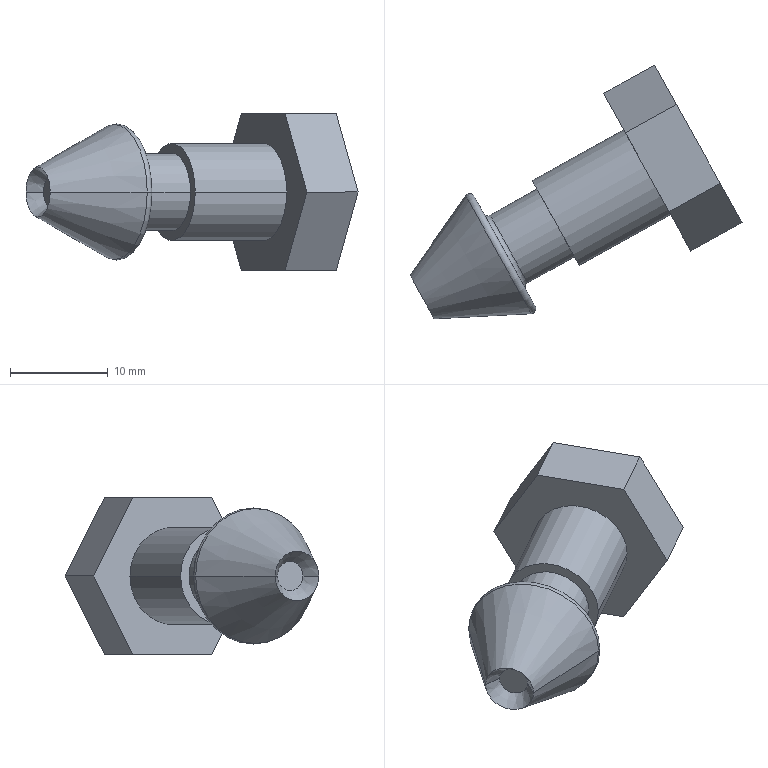Part | STEP file | Completa.sldasm-Part-30_Valor predeterminado | 1 solid | 23 faces | box 34.045 x 26.016 x 16 mm | volume 3225 mm3 | plane 11 | torus 4 | cone 4 | cylinder 4 | commonest cylinder face diameters 7.936 x2 9.938 x2
STEP:
#1=CARTESIAN_POINT('',(0.,0.,0.));
#2=DIRECTION('',(0.,0.,1.));
#3=DIRECTION('',(1.,0.,0.));
#4=AXIS2_PLACEMENT_3D('',#1,#2,#3);
#5=CARTESIAN_POINT('',(-90.416,128.396,0.));
#6=VERTEX_POINT('',#5);
#7=CARTESIAN_POINT('',(-97.128,140.507,0.));
#8=VERTEX_POINT('',#7);
#9=CARTESIAN_POINT('',(-93.772,134.451,0.));
#10=DIRECTION('',(-0.8747,-0.4847,0.));
#11=DIRECTION('',(0.4847,-0.8747,0.));
#12=AXIS2_PLACEMENT_3D('',#9,#10,#11);
#13=CIRCLE('',#12,6.924);
#14=CARTESIAN_POINT('',(-93.58,134.558,0.));
#15=DIRECTION('',(0.8747,0.4847,0.));
#16=DIRECTION('',(-0.4847,0.8747,0.));
#17=AXIS2_PLACEMENT_3D('',#14,#15,#16);
#18=TOROIDAL_SURFACE('',#17,6.474,0.5);
#19=CARTESIAN_POINT('',(3.142,-0.4538));
#20=DIRECTION('',(-1.,0.));
#21=VECTOR('',#20,1.);
#22=LINE('',#19,#21);
#23=(GEOMETRIC_REPRESENTATION_CONTEXT(2)PARAMETRIC_REPRESENTATION_CONTEXT()REPRESENTATION_CONTEXT('',''));
#24=DEFINITIONAL_REPRESENTATION('',(#22),#23);
#25=PCURVE('',#18,#24);
#26=CARTESIAN_POINT('',(-101.601,130.113,0.));
#27=DIRECTION('',(0.8747,0.4847,0.));
#28=DIRECTION('',(-0.4847,0.8747,0.));
#29=AXIS2_PLACEMENT_3D('',#26,#27,#28);
#30=CONICAL_SURFACE('',#29,2.558,0.4538);
#31=CARTESIAN_POINT('',(3.142,8.951));
#32=DIRECTION('',(-1.,0.));
#33=VECTOR('',#32,1.);
#34=LINE('',#31,#33);
#35=(GEOMETRIC_REPRESENTATION_CONTEXT(2)PARAMETRIC_REPRESENTATION_CONTEXT()REPRESENTATION_CONTEXT('',''));
#36=DEFINITIONAL_REPRESENTATION('',(#34),#35);
#37=PCURVE('',#30,#36);
#38=SURFACE_CURVE('',#13,(#25,#37),.PCURVE_S1.);
#39=EDGE_CURVE('',#6,#8,#38,.T.);
#40=ORIENTED_EDGE('',*,*,#39,.F.);
#41=CARTESIAN_POINT('',(-90.004,129.137,0.));
#42=VERTEX_POINT('',#41);
#43=CARTESIAN_POINT('',(-90.442,128.895,0.));
#44=DIRECTION('',(0.,0.,1.));
#45=DIRECTION('',(0.,-1.,0.));
#46=AXIS2_PLACEMENT_3D('',#43,#44,#45);
#47=CIRCLE('',#46,0.5);
#48=CARTESIAN_POINT('',(3.142,-0.5061));
#49=DIRECTION('',(0.,1.));
#50=VECTOR('',#49,1.);
#51=LINE('',#48,#50);
#52=(GEOMETRIC_REPRESENTATION_CONTEXT(2)PARAMETRIC_REPRESENTATION_CONTEXT()REPRESENTATION_CONTEXT('',''));
#53=DEFINITIONAL_REPRESENTATION('',(#51),#52);
#54=PCURVE('',#18,#53);
#55=CARTESIAN_POINT('',(-93.58,134.558,0.));
#56=DIRECTION('',(0.8747,0.4847,0.));
#57=DIRECTION('',(-0.4847,0.8747,0.));
#58=AXIS2_PLACEMENT_3D('',#55,#56,#57);
#59=TOROIDAL_SURFACE('',#58,6.474,0.5);
#60=CARTESIAN_POINT('',(3.142,-0.5061));
#61=DIRECTION('',(0.,1.));
#62=VECTOR('',#61,1.);
#63=LINE('',#60,#62);
#64=(GEOMETRIC_REPRESENTATION_CONTEXT(2)PARAMETRIC_REPRESENTATION_CONTEXT()REPRESENTATION_CONTEXT('',''));
#65=DEFINITIONAL_REPRESENTATION('',(#63),#64);
#66=PCURVE('',#59,#65);
#67=SURFACE_CURVE('',#47,(#54,#66),.PCURVE_S1.);
#68=EDGE_CURVE('',#6,#42,#67,.T.);
#69=ORIENTED_EDGE('',*,*,#68,.T.);
#70=CARTESIAN_POINT('',(-96.281,140.463,0.));
#71=VERTEX_POINT('',#70);
#72=CARTESIAN_POINT('',(-93.143,134.8,0.));
#73=DIRECTION('',(0.8747,0.4847,0.));
#74=DIRECTION('',(-0.4847,0.8747,0.));
#75=AXIS2_PLACEMENT_3D('',#72,#73,#74);
#76=CIRCLE('',#75,6.474);
#77=CARTESIAN_POINT('',(0.,1.571));
#78=DIRECTION('',(1.,0.));
#79=VECTOR('',#78,1.);
#80=LINE('',#77,#79);
#81=(GEOMETRIC_REPRESENTATION_CONTEXT(2)PARAMETRIC_REPRESENTATION_CONTEXT()REPRESENTATION_CONTEXT('',''));
#82=DEFINITIONAL_REPRESENTATION('',(#80),#81);
#83=PCURVE('',#18,#82);
#84=CARTESIAN_POINT('',(-96.669,141.163,0.));
#85=DIRECTION('',(0.8747,0.4847,0.));
#86=DIRECTION('',(-0.4847,0.8747,0.));
#87=AXIS2_PLACEMENT_3D('',#84,#85,#86);
#88=PLANE('',#87);
#89=CARTESIAN_POINT('',(-7.274,0.));
#90=DIRECTION('',(1.,0.));
#91=AXIS2_PLACEMENT_2D('',#89,#90);
#92=CIRCLE('',#91,6.474);
#93=(GEOMETRIC_REPRESENTATION_CONTEXT(2)PARAMETRIC_REPRESENTATION_CONTEXT()REPRESENTATION_CONTEXT('',''));
#94=DEFINITIONAL_REPRESENTATION('',(#92),#93);
#95=PCURVE('',#88,#94);
#96=SURFACE_CURVE('',#76,(#83,#95),.PCURVE_S1.);
#97=EDGE_CURVE('',#71,#42,#96,.T.);
#98=ORIENTED_EDGE('',*,*,#97,.F.);
#99=CARTESIAN_POINT('',(-96.718,140.22,0.));
#100=DIRECTION('',(0.,0.,-1.));
#101=DIRECTION('',(-1.,0.,0.));
#102=AXIS2_PLACEMENT_3D('',#99,#100,#101);
#103=CIRCLE('',#102,0.5);
#104=CARTESIAN_POINT('',(0.,-1.065));
#105=DIRECTION('',(0.,1.));
#106=VECTOR('',#105,1.);
#107=LINE('',#104,#106);
#108=(GEOMETRIC_REPRESENTATION_CONTEXT(2)PARAMETRIC_REPRESENTATION_CONTEXT()REPRESENTATION_CONTEXT('',''));
#109=DEFINITIONAL_REPRESENTATION('',(#107),#108);
#110=PCURVE('',#18,#109);
#111=CARTESIAN_POINT('',(6.283,-1.065));
#112=DIRECTION('',(0.,1.));
#113=VECTOR('',#112,1.);
#114=LINE('',#111,#113);
#115=(GEOMETRIC_REPRESENTATION_CONTEXT(2)PARAMETRIC_REPRESENTATION_CONTEXT()REPRESENTATION_CONTEXT('',''));
#116=DEFINITIONAL_REPRESENTATION('',(#114),#115);
#117=PCURVE('',#59,#116);
#118=SURFACE_CURVE('',#103,(#110,#117),.PCURVE_S1.);
#119=EDGE_CURVE('',#8,#71,#118,.T.);
#120=ORIENTED_EDGE('',*,*,#119,.F.);
#121=EDGE_LOOP('',(#40,#69,#98,#120));
#122=FACE_BOUND('',#121,.T.);
#123=ADVANCED_FACE('',(#122),#18,.T.);
#124=CARTESIAN_POINT('',(-94.629,138.513,0.));
#125=VERTEX_POINT('',#124);
#126=CARTESIAN_POINT('',(-95.309,138.708,0.));
#127=VERTEX_POINT('',#126);
#128=CARTESIAN_POINT('',(-94.871,138.95,0.));
#129=DIRECTION('',(0.,0.,-1.));
#130=DIRECTION('',(-1.,0.,0.));
#131=AXIS2_PLACEMENT_3D('',#128,#129,#130);
#132=CIRCLE('',#131,0.5);
#133=CARTESIAN_POINT('',(-92.705,135.042,0.));
#134=DIRECTION('',(0.8747,0.4847,0.));
#135=DIRECTION('',(-0.4847,0.8747,0.));
#136=AXIS2_PLACEMENT_3D('',#133,#134,#135);
#137=TOROIDAL_SURFACE('',#136,4.468,0.5);
#138=CARTESIAN_POINT('',(6.283,-1.065));
#139=DIRECTION('',(0.,1.));
#140=VECTOR('',#139,1.);
#141=LINE('',#138,#140);
#142=(GEOMETRIC_REPRESENTATION_CONTEXT(2)PARAMETRIC_REPRESENTATION_CONTEXT()REPRESENTATION_CONTEXT('',''));
#143=DEFINITIONAL_REPRESENTATION('',(#141),#142);
#144=PCURVE('',#137,#143);
#145=CARTESIAN_POINT('',(-92.705,135.042,0.));
#146=DIRECTION('',(0.8747,0.4847,0.));
#147=DIRECTION('',(-0.4847,0.8747,0.));
#148=AXIS2_PLACEMENT_3D('',#145,#146,#147);
#149=TOROIDAL_SURFACE('',#148,4.468,0.5);
#150=CARTESIAN_POINT('',(0.,-1.065));
#151=DIRECTION('',(0.,1.));
#152=VECTOR('',#151,1.);
#153=LINE('',#150,#152);
#154=(GEOMETRIC_REPRESENTATION_CONTEXT(2)PARAMETRIC_REPRESENTATION_CONTEXT()REPRESENTATION_CONTEXT('',''));
#155=DEFINITIONAL_REPRESENTATION('',(#153),#154);
#156=PCURVE('',#149,#155);
#157=SURFACE_CURVE('',#132,(#144,#156),.PCURVE_S1.);
#158=EDGE_CURVE('',#125,#127,#157,.T.);
#159=ORIENTED_EDGE('',*,*,#158,.T.);
#160=CARTESIAN_POINT('',(-90.977,130.892,0.));
#161=VERTEX_POINT('',#160);
#162=CARTESIAN_POINT('',(-93.143,134.8,0.));
#163=DIRECTION('',(-0.8747,-0.4847,0.));
#164=DIRECTION('',(-0.4847,0.8747,0.));
#165=AXIS2_PLACEMENT_3D('',#162,#163,#164);
#166=CIRCLE('',#165,4.468);
#167=CARTESIAN_POINT('',(6.283,4.712));
#168=DIRECTION('',(-1.,0.));
#169=VECTOR('',#168,1.);
#170=LINE('',#167,#169);
#171=(GEOMETRIC_REPRESENTATION_CONTEXT(2)PARAMETRIC_REPRESENTATION_CONTEXT()REPRESENTATION_CONTEXT('',''));
#172=DEFINITIONAL_REPRESENTATION('',(#170),#171);
#173=PCURVE('',#137,#172);
#174=CARTESIAN_POINT('',(-2.806,0.));
#175=CARTESIAN_POINT('',(-2.806,-7.739));
#176=CARTESIAN_POINT('',(-9.508,-3.87));
#177=CARTESIAN_POINT('',(-16.211,0.));
#178=CARTESIAN_POINT('',(-9.508,3.87));
#179=CARTESIAN_POINT('',(-2.806,7.739));
#180=CARTESIAN_POINT('',(-2.806,0.));
#181=(BOUNDED_CURVE()B_SPLINE_CURVE(2,(#174,#175,#176,#177,#178,#179,#180),.UNSPECIFIED.,.T.,.F.)B_SPLINE_CURVE_WITH_KNOTS((1,2,2,2,2,1),(-2.094,0.,2.094,4.189,6.283,8.378),.UNSPECIFIED.)CURVE()GEOMETRIC_REPRESENTATION_ITEM()RATIONAL_B_SPLINE_CURVE((1.,0.5,1.,0.5,1.,0.5,1.))REPRESENTATION_ITEM(''));
#182=(GEOMETRIC_REPRESENTATION_CONTEXT(2)PARAMETRIC_REPRESENTATION_CONTEXT()REPRESENTATION_CONTEXT('',''));
#183=DEFINITIONAL_REPRESENTATION('',(#181),#182);
#184=PCURVE('',#88,#183);
#185=SURFACE_CURVE('',#166,(#173,#184),.PCURVE_S1.);
#186=EDGE_CURVE('',#127,#161,#185,.T.);
#187=ORIENTED_EDGE('',*,*,#186,.T.);
#188=CARTESIAN_POINT('',(-90.782,131.571,0.));
#189=VERTEX_POINT('',#188);
#190=CARTESIAN_POINT('',(-90.54,131.134,0.));
#191=DIRECTION('',(0.,0.,1.));
#192=DIRECTION('',(0.,-1.,0.));
#193=AXIS2_PLACEMENT_3D('',#190,#191,#192);
#194=CIRCLE('',#193,0.5);
#195=CARTESIAN_POINT('',(3.142,-0.5061));
#196=DIRECTION('',(0.,1.));
#197=VECTOR('',#196,1.);
#198=LINE('',#195,#197);
#199=(GEOMETRIC_REPRESENTATION_CONTEXT(2)PARAMETRIC_REPRESENTATION_CONTEXT()REPRESENTATION_CONTEXT('',''));
#200=DEFINITIONAL_REPRESENTATION('',(#198),#199);
#201=PCURVE('',#137,#200);
#202=CARTESIAN_POINT('',(3.142,-0.5061));
#203=DIRECTION('',(0.,1.));
#204=VECTOR('',#203,1.);
#205=LINE('',#202,#204);
#206=(GEOMETRIC_REPRESENTATION_CONTEXT(2)PARAMETRIC_REPRESENTATION_CONTEXT()REPRESENTATION_CONTEXT('',''));
#207=DEFINITIONAL_REPRESENTATION('',(#205),#206);
#208=PCURVE('',#149,#207);
#209=SURFACE_CURVE('',#194,(#201,#208),.PCURVE_S1.);
#210=EDGE_CURVE('',#189,#161,#209,.T.);
#211=ORIENTED_EDGE('',*,*,#210,.F.);
#212=CARTESIAN_POINT('',(-92.705,135.042,0.));
#213=DIRECTION('',(0.8747,0.4847,0.));
#214=DIRECTION('',(-0.4847,0.8747,0.));
#215=AXIS2_PLACEMENT_3D('',#212,#213,#214);
#216=CIRCLE('',#215,3.968);
#217=CARTESIAN_POINT('',(0.,3.142));
#218=DIRECTION('',(1.,0.));
#219=VECTOR('',#218,1.);
#220=LINE('',#217,#219);
#221=(GEOMETRIC_REPRESENTATION_CONTEXT(2)PARAMETRIC_REPRESENTATION_CONTEXT()REPRESENTATION_CONTEXT('',''));
#222=DEFINITIONAL_REPRESENTATION('',(#220),#221);
#223=PCURVE('',#137,#222);
#224=CARTESIAN_POINT('',(-81.185,141.427,0.));
#225=DIRECTION('',(-0.8747,-0.4847,0.));
#226=DIRECTION('',(0.4847,-0.8747,0.));
#227=AXIS2_PLACEMENT_3D('',#224,#225,#226);
#228=CYLINDRICAL_SURFACE('',#227,3.968);
#229=CARTESIAN_POINT('',(9.425,13.172));
#230=DIRECTION('',(-1.,0.));
#231=VECTOR('',#230,1.);
#232=LINE('',#229,#231);
#233=(GEOMETRIC_REPRESENTATION_CONTEXT(2)PARAMETRIC_REPRESENTATION_CONTEXT()REPRESENTATION_CONTEXT('',''));
#234=DEFINITIONAL_REPRESENTATION('',(#232),#233);
#235=PCURVE('',#228,#234);
#236=SURFACE_CURVE('',#216,(#223,#235),.PCURVE_S1.);
#237=EDGE_CURVE('',#189,#125,#236,.T.);
#238=ORIENTED_EDGE('',*,*,#237,.T.);
#239=EDGE_LOOP('',(#159,#187,#211,#238));
#240=FACE_BOUND('',#239,.F.);
#241=ADVANCED_FACE('',(#240),#137,.F.);
#242=CARTESIAN_POINT('',(-99.6,129.506,0.));
#243=VERTEX_POINT('',#242);
#244=CARTESIAN_POINT('',(-100.361,127.875,0.));
#245=VERTEX_POINT('',#244);
#246=CARTESIAN_POINT('',(-99.6,129.506,0.));
#247=DIRECTION('',(-0.4227,-0.9063,0.));
#248=VECTOR('',#247,1.);
#249=LINE('',#246,#248);
#250=CARTESIAN_POINT('',(-100.327,130.818,0.));
#251=DIRECTION('',(-0.8747,-0.4847,0.));
#252=DIRECTION('',(0.4847,-0.8747,0.));
#253=AXIS2_PLACEMENT_3D('',#250,#251,#252);
#254=CONICAL_SURFACE('',#253,1.5,0.6283);
#255=CARTESIAN_POINT('',(6.283,0.));
#256=DIRECTION('',(0.,1.));
#257=VECTOR('',#256,1.);
#258=LINE('',#255,#257);
#259=(GEOMETRIC_REPRESENTATION_CONTEXT(2)PARAMETRIC_REPRESENTATION_CONTEXT()REPRESENTATION_CONTEXT('',''));
#260=DEFINITIONAL_REPRESENTATION('',(#258),#259);
#261=PCURVE('',#254,#260);
#262=CARTESIAN_POINT('',(-100.327,130.818,0.));
#263=DIRECTION('',(-0.8747,-0.4847,0.));
#264=DIRECTION('',(0.4847,-0.8747,0.));
#265=AXIS2_PLACEMENT_3D('',#262,#263,#264);
#266=CONICAL_SURFACE('',#265,1.5,0.6283);
#267=CARTESIAN_POINT('',(0.,0.));
#268=DIRECTION('',(0.,1.));
#269=VECTOR('',#268,1.);
#270=LINE('',#267,#269);
#271=(GEOMETRIC_REPRESENTATION_CONTEXT(2)PARAMETRIC_REPRESENTATION_CONTEXT()REPRESENTATION_CONTEXT('',''));
#272=DEFINITIONAL_REPRESENTATION('',(#270),#271);
#273=PCURVE('',#266,#272);
#274=SURFACE_CURVE('',#249,(#261,#273),.PCURVE_S1.);
#275=EDGE_CURVE('',#243,#245,#274,.T.);
#276=ORIENTED_EDGE('',*,*,#275,.T.);
#277=CARTESIAN_POINT('',(-102.841,132.35,0.));
#278=VERTEX_POINT('',#277);
#279=CARTESIAN_POINT('',(-101.601,130.113,0.));
#280=DIRECTION('',(-0.8747,-0.4847,0.));
#281=DIRECTION('',(0.4847,-0.8747,0.));
#282=AXIS2_PLACEMENT_3D('',#279,#280,#281);
#283=CIRCLE('',#282,2.558);
#284=CARTESIAN_POINT('',(0.,1.456));
#285=DIRECTION('',(1.,0.));
#286=VECTOR('',#285,1.);
#287=LINE('',#284,#286);
#288=(GEOMETRIC_REPRESENTATION_CONTEXT(2)PARAMETRIC_REPRESENTATION_CONTEXT()REPRESENTATION_CONTEXT('',''));
#289=DEFINITIONAL_REPRESENTATION('',(#287),#288);
#290=PCURVE('',#254,#289);
#291=CARTESIAN_POINT('',(-101.601,130.113,0.));
#292=DIRECTION('',(0.8747,0.4847,0.));
#293=DIRECTION('',(-0.4847,0.8747,0.));
#294=AXIS2_PLACEMENT_3D('',#291,#292,#293);
#295=CONICAL_SURFACE('',#294,2.558,0.4538);
#296=CARTESIAN_POINT('',(9.425,0.));
#297=DIRECTION('',(-1.,0.));
#298=VECTOR('',#297,1.);
#299=LINE('',#296,#298);
#300=(GEOMETRIC_REPRESENTATION_CONTEXT(2)PARAMETRIC_REPRESENTATION_CONTEXT()REPRESENTATION_CONTEXT('',''));
#301=DEFINITIONAL_REPRESENTATION('',(#299),#300);
#302=PCURVE('',#295,#301);
#303=SURFACE_CURVE('',#283,(#290,#302),.PCURVE_S1.);
#304=EDGE_CURVE('',#278,#245,#303,.T.);
#305=ORIENTED_EDGE('',*,*,#304,.F.);
#306=CARTESIAN_POINT('',(-101.054,132.13,0.));
#307=VERTEX_POINT('',#306);
#308=CARTESIAN_POINT('',(-101.054,132.13,0.));
#309=DIRECTION('',(-0.9925,0.122,0.));
#310=VECTOR('',#309,1.);
#311=LINE('',#308,#310);
#312=CARTESIAN_POINT('',(3.142,0.));
#313=DIRECTION('',(0.,1.));
#314=VECTOR('',#313,1.);
#315=LINE('',#312,#314);
#316=(GEOMETRIC_REPRESENTATION_CONTEXT(2)PARAMETRIC_REPRESENTATION_CONTEXT()REPRESENTATION_CONTEXT('',''));
#317=DEFINITIONAL_REPRESENTATION('',(#315),#316);
#318=PCURVE('',#254,#317);
#319=CARTESIAN_POINT('',(3.142,0.));
#320=DIRECTION('',(0.,1.));
#321=VECTOR('',#320,1.);
#322=LINE('',#319,#321);
#323=(GEOMETRIC_REPRESENTATION_CONTEXT(2)PARAMETRIC_REPRESENTATION_CONTEXT()REPRESENTATION_CONTEXT('',''));
#324=DEFINITIONAL_REPRESENTATION('',(#322),#323);
#325=PCURVE('',#266,#324);
#326=SURFACE_CURVE('',#311,(#318,#325),.PCURVE_S1.);
#327=EDGE_CURVE('',#307,#278,#326,.T.);
#328=ORIENTED_EDGE('',*,*,#327,.F.);
#329=CARTESIAN_POINT('',(-100.327,130.818,0.));
#330=DIRECTION('',(-0.8747,-0.4847,0.));
#331=DIRECTION('',(0.4847,-0.8747,0.));
#332=AXIS2_PLACEMENT_3D('',#329,#330,#331);
#333=CIRCLE('',#332,1.5);
#334=CARTESIAN_POINT('',(0.,0.));
#335=DIRECTION('',(1.,0.));
#336=VECTOR('',#335,1.);
#337=LINE('',#334,#336);
#338=(GEOMETRIC_REPRESENTATION_CONTEXT(2)PARAMETRIC_REPRESENTATION_CONTEXT()REPRESENTATION_CONTEXT('',''));
#339=DEFINITIONAL_REPRESENTATION('',(#337),#338);
#340=PCURVE('',#254,#339);
#341=CARTESIAN_POINT('',(-100.327,130.818,0.));
#342=DIRECTION('',(-0.8747,-0.4847,0.));
#343=DIRECTION('',(0.4847,-0.8747,0.));
#344=AXIS2_PLACEMENT_3D('',#341,#342,#343);
#345=PLANE('',#344);
#346=CARTESIAN_POINT('',(0.,0.));
#347=DIRECTION('',(1.,0.));
#348=AXIS2_PLACEMENT_2D('',#346,#347);
#349=CIRCLE('',#348,1.5);
#350=(GEOMETRIC_REPRESENTATION_CONTEXT(2)PARAMETRIC_REPRESENTATION_CONTEXT()REPRESENTATION_CONTEXT('',''));
#351=DEFINITIONAL_REPRESENTATION('',(#349),#350);
#352=PCURVE('',#345,#351);
#353=SURFACE_CURVE('',#333,(#340,#352),.PCURVE_S1.);
#354=EDGE_CURVE('',#307,#243,#353,.T.);
#355=ORIENTED_EDGE('',*,*,#354,.T.);
#356=EDGE_LOOP('',(#276,#305,#328,#355));
#357=FACE_BOUND('',#356,.F.);
#358=ADVANCED_FACE('',(#357),#254,.F.);
#359=CARTESIAN_POINT('',(-101.601,130.113,0.));
#360=DIRECTION('',(-0.8747,-0.4847,0.));
#361=DIRECTION('',(0.4847,-0.8747,0.));
#362=AXIS2_PLACEMENT_3D('',#359,#360,#361);
#363=CIRCLE('',#362,2.558);
#364=CARTESIAN_POINT('',(3.142,0.));
#365=DIRECTION('',(-1.,0.));
#366=VECTOR('',#365,1.);
#367=LINE('',#364,#366);
#368=(GEOMETRIC_REPRESENTATION_CONTEXT(2)PARAMETRIC_REPRESENTATION_CONTEXT()REPRESENTATION_CONTEXT('',''));
#369=DEFINITIONAL_REPRESENTATION('',(#367),#368);
#370=PCURVE('',#30,#369);
#371=CARTESIAN_POINT('',(0.,1.456));
#372=DIRECTION('',(1.,0.));
#373=VECTOR('',#372,1.);
#374=LINE('',#371,#373);
#375=(GEOMETRIC_REPRESENTATION_CONTEXT(2)PARAMETRIC_REPRESENTATION_CONTEXT()REPRESENTATION_CONTEXT('',''));
#376=DEFINITIONAL_REPRESENTATION('',(#374),#375);
#377=PCURVE('',#266,#376);
#378=SURFACE_CURVE('',#363,(#370,#377),.PCURVE_S1.);
#379=EDGE_CURVE('',#245,#278,#378,.T.);
#380=ORIENTED_EDGE('',*,*,#379,.F.);
#381=CARTESIAN_POINT('',(-100.361,127.875,0.));
#382=DIRECTION('',(0.9986,0.05225,0.));
#383=VECTOR('',#382,1.);
#384=LINE('',#381,#383);
#385=CARTESIAN_POINT('',(3.142,0.));
#386=DIRECTION('',(0.,1.));
#387=VECTOR('',#386,1.);
#388=LINE('',#385,#387);
#389=(GEOMETRIC_REPRESENTATION_CONTEXT(2)PARAMETRIC_REPRESENTATION_CONTEXT()REPRESENTATION_CONTEXT('',''));
#390=DEFINITIONAL_REPRESENTATION('',(#388),#389);
#391=PCURVE('',#30,#390);
#392=CARTESIAN_POINT('',(3.142,0.));
#393=DIRECTION('',(0.,1.));
#394=VECTOR('',#393,1.);
#395=LINE('',#392,#394);
#396=(GEOMETRIC_REPRESENTATION_CONTEXT(2)PARAMETRIC_REPRESENTATION_CONTEXT()REPRESENTATION_CONTEXT('',''));
#397=DEFINITIONAL_REPRESENTATION('',(#395),#396);
#398=PCURVE('',#295,#397);
#399=SURFACE_CURVE('',#384,(#391,#398),.PCURVE_S1.);
#400=EDGE_CURVE('',#245,#6,#399,.T.);
#401=ORIENTED_EDGE('',*,*,#400,.T.);
#402=ORIENTED_EDGE('',*,*,#39,.T.);
#403=CARTESIAN_POINT('',(-102.841,132.35,0.));
#404=DIRECTION('',(0.5736,0.8191,0.));
#405=VECTOR('',#404,1.);
#406=LINE('',#403,#405);
#407=CARTESIAN_POINT('',(0.,0.));
#408=DIRECTION('',(0.,1.));
#409=VECTOR('',#408,1.);
#410=LINE('',#407,#409);
#411=(GEOMETRIC_REPRESENTATION_CONTEXT(2)PARAMETRIC_REPRESENTATION_CONTEXT()REPRESENTATION_CONTEXT('',''));
#412=DEFINITIONAL_REPRESENTATION('',(#410),#411);
#413=PCURVE('',#30,#412);
#414=CARTESIAN_POINT('',(6.283,0.));
#415=DIRECTION('',(0.,1.));
#416=VECTOR('',#415,1.);
#417=LINE('',#414,#416);
#418=(GEOMETRIC_REPRESENTATION_CONTEXT(2)PARAMETRIC_REPRESENTATION_CONTEXT()REPRESENTATION_CONTEXT('',''));
#419=DEFINITIONAL_REPRESENTATION('',(#417),#418);
#420=PCURVE('',#295,#419);
#421=SURFACE_CURVE('',#406,(#413,#420),.PCURVE_S1.);
#422=EDGE_CURVE('',#278,#8,#421,.T.);
#423=ORIENTED_EDGE('',*,*,#422,.F.);
#424=EDGE_LOOP('',(#380,#401,#402,#423));
#425=FACE_BOUND('',#424,.T.);
#426=ADVANCED_FACE('',(#425),#30,.T.);
#427=CARTESIAN_POINT('',(-85.971,134.238,0.));
#428=VERTEX_POINT('',#427);
#429=CARTESIAN_POINT('',(-89.818,141.179,0.));
#430=VERTEX_POINT('',#429);
#431=CARTESIAN_POINT('',(-87.895,137.708,0.));
#432=DIRECTION('',(-0.8747,-0.4847,0.));
#433=DIRECTION('',(0.4847,-0.8747,0.));
#434=AXIS2_PLACEMENT_3D('',#431,#432,#433);
#435=CIRCLE('',#434,3.968);
#436=CARTESIAN_POINT('',(-81.185,141.427,0.));
#437=DIRECTION('',(-0.8747,-0.4847,0.));
#438=DIRECTION('',(0.4847,-0.8747,0.));
#439=AXIS2_PLACEMENT_3D('',#436,#437,#438);
#440=CYLINDRICAL_SURFACE('',#439,3.968);
#441=CARTESIAN_POINT('',(0.,7.672));
#442=DIRECTION('',(1.,0.));
#443=VECTOR('',#442,1.);
#444=LINE('',#441,#443);
#445=(GEOMETRIC_REPRESENTATION_CONTEXT(2)PARAMETRIC_REPRESENTATION_CONTEXT()REPRESENTATION_CONTEXT('',''));
#446=DEFINITIONAL_REPRESENTATION('',(#444),#445);
#447=PCURVE('',#440,#446);
#448=CARTESIAN_POINT('',(-89.818,141.179,0.));
#449=DIRECTION('',(-0.8747,-0.4847,0.));
#450=DIRECTION('',(0.4847,-0.8747,0.));
#451=AXIS2_PLACEMENT_3D('',#448,#449,#450);
#452=PLANE('',#451);
#453=CARTESIAN_POINT('',(3.968,0.));
#454=DIRECTION('',(1.,0.));
#455=AXIS2_PLACEMENT_2D('',#453,#454);
#456=CIRCLE('',#455,3.968);
#457=(GEOMETRIC_REPRESENTATION_CONTEXT(2)PARAMETRIC_REPRESENTATION_CONTEXT()REPRESENTATION_CONTEXT('',''));
#458=DEFINITIONAL_REPRESENTATION('',(#456),#457);
#459=PCURVE('',#452,#458);
#460=SURFACE_CURVE('',#435,(#447,#459),.PCURVE_S1.);
#461=EDGE_CURVE('',#428,#430,#460,.T.);
#462=ORIENTED_EDGE('',*,*,#461,.T.);
#463=CARTESIAN_POINT('',(-83.108,144.898,0.));
#464=DIRECTION('',(-0.8747,-0.4847,0.));
#465=VECTOR('',#464,1.);
#466=LINE('',#463,#465);
#467=CARTESIAN_POINT('',(3.142,0.));
#468=DIRECTION('',(0.,1.));
#469=VECTOR('',#468,1.);
#470=LINE('',#467,#469);
#471=(GEOMETRIC_REPRESENTATION_CONTEXT(2)PARAMETRIC_REPRESENTATION_CONTEXT()REPRESENTATION_CONTEXT('',''));
#472=DEFINITIONAL_REPRESENTATION('',(#470),#471);
#473=PCURVE('',#440,#472);
#474=CARTESIAN_POINT('',(3.142,0.));
#475=DIRECTION('',(0.,1.));
#476=VECTOR('',#475,1.);
#477=LINE('',#474,#476);
#478=(GEOMETRIC_REPRESENTATION_CONTEXT(2)PARAMETRIC_REPRESENTATION_CONTEXT()REPRESENTATION_CONTEXT('',''));
#479=DEFINITIONAL_REPRESENTATION('',(#477),#478);
#480=PCURVE('',#228,#479);
#481=SURFACE_CURVE('',#466,(#473,#480),.PCURVE_S1.);
#482=EDGE_CURVE('',#430,#125,#481,.T.);
#483=ORIENTED_EDGE('',*,*,#482,.T.);
#484=CARTESIAN_POINT('',(-92.705,135.042,0.));
#485=DIRECTION('',(0.8747,0.4847,0.));
#486=DIRECTION('',(-0.4847,0.8747,0.));
#487=AXIS2_PLACEMENT_3D('',#484,#485,#486);
#488=CIRCLE('',#487,3.968);
#489=CARTESIAN_POINT('',(3.142,13.172));
#490=DIRECTION('',(-1.,0.));
#491=VECTOR('',#490,1.);
#492=LINE('',#489,#491);
#493=(GEOMETRIC_REPRESENTATION_CONTEXT(2)PARAMETRIC_REPRESENTATION_CONTEXT()REPRESENTATION_CONTEXT('',''));
#494=DEFINITIONAL_REPRESENTATION('',(#492),#493);
#495=PCURVE('',#440,#494);
#496=CARTESIAN_POINT('',(0.,3.142));
#497=DIRECTION('',(1.,0.));
#498=VECTOR('',#497,1.);
#499=LINE('',#496,#498);
#500=(GEOMETRIC_REPRESENTATION_CONTEXT(2)PARAMETRIC_REPRESENTATION_CONTEXT()REPRESENTATION_CONTEXT('',''));
#501=DEFINITIONAL_REPRESENTATION('',(#499),#500);
#502=PCURVE('',#149,#501);
#503=SURFACE_CURVE('',#488,(#495,#502),.PCURVE_S1.);
#504=EDGE_CURVE('',#125,#189,#503,.T.);
#505=ORIENTED_EDGE('',*,*,#504,.T.);
#506=CARTESIAN_POINT('',(-79.261,137.956,0.));
#507=DIRECTION('',(-0.8747,-0.4847,0.));
#508=VECTOR('',#507,1.);
#509=LINE('',#506,#508);
#510=CARTESIAN_POINT('',(0.,0.));
#511=DIRECTION('',(0.,1.));
#512=VECTOR('',#511,1.);
#513=LINE('',#510,#512);
#514=(GEOMETRIC_REPRESENTATION_CONTEXT(2)PARAMETRIC_REPRESENTATION_CONTEXT()REPRESENTATION_CONTEXT('',''));
#515=DEFINITIONAL_REPRESENTATION('',(#513),#514);
#516=PCURVE('',#440,#515);
#517=CARTESIAN_POINT('',(6.283,0.));
#518=DIRECTION('',(0.,1.));
#519=VECTOR('',#518,1.);
#520=LINE('',#517,#519);
#521=(GEOMETRIC_REPRESENTATION_CONTEXT(2)PARAMETRIC_REPRESENTATION_CONTEXT()REPRESENTATION_CONTEXT('',''));
#522=DEFINITIONAL_REPRESENTATION('',(#520),#521);
#523=PCURVE('',#228,#522);
#524=SURFACE_CURVE('',#509,(#516,#523),.PCURVE_S1.);
#525=EDGE_CURVE('',#428,#189,#524,.T.);
#526=ORIENTED_EDGE('',*,*,#525,.F.);
#527=EDGE_LOOP('',(#462,#483,#505,#526));
#528=FACE_BOUND('',#527,.T.);
#529=ADVANCED_FACE('',(#528),#440,.T.);
#530=CARTESIAN_POINT('',(-76.112,138.557,0.));
#531=VERTEX_POINT('',#530);
#532=CARTESIAN_POINT('',(-80.93,147.249,0.));
#533=VERTEX_POINT('',#532);
#534=CARTESIAN_POINT('',(-78.521,142.903,0.));
#535=DIRECTION('',(-0.8747,-0.4847,0.));
#536=DIRECTION('',(0.4847,-0.8747,0.));
#537=AXIS2_PLACEMENT_3D('',#534,#535,#536);
#538=CIRCLE('',#537,4.969);
#539=CARTESIAN_POINT('',(-81.185,141.427,0.));
#540=DIRECTION('',(-0.8747,-0.4847,0.));
#541=DIRECTION('',(0.4847,-0.8747,0.));
#542=AXIS2_PLACEMENT_3D('',#539,#540,#541);
#543=CYLINDRICAL_SURFACE('',#542,4.969);
#544=CARTESIAN_POINT('',(0.,-3.045));
#545=DIRECTION('',(1.,0.));
#546=VECTOR('',#545,1.);
#547=LINE('',#544,#546);
#548=(GEOMETRIC_REPRESENTATION_CONTEXT(2)PARAMETRIC_REPRESENTATION_CONTEXT()REPRESENTATION_CONTEXT('',''));
#549=DEFINITIONAL_REPRESENTATION('',(#547),#548);
#550=PCURVE('',#543,#549);
#551=CARTESIAN_POINT('',(-74.043,134.823,0.));
#552=DIRECTION('',(-0.8747,-0.4847,0.));
#553=DIRECTION('',(0.4847,-0.8747,0.));
#554=AXIS2_PLACEMENT_3D('',#551,#552,#553);
#555=PLANE('',#554);
#556=CARTESIAN_POINT('',(-9.238,0.));
#557=DIRECTION('',(1.,0.));
#558=AXIS2_PLACEMENT_2D('',#556,#557);
#559=CIRCLE('',#558,4.969);
#560=(GEOMETRIC_REPRESENTATION_CONTEXT(2)PARAMETRIC_REPRESENTATION_CONTEXT()REPRESENTATION_CONTEXT('',''));
#561=DEFINITIONAL_REPRESENTATION('',(#559),#560);
#562=PCURVE('',#555,#561);
#563=SURFACE_CURVE('',#538,(#550,#562),.PCURVE_S1.);
#564=EDGE_CURVE('',#531,#533,#563,.T.);
#565=ORIENTED_EDGE('',*,*,#564,.T.);
#566=CARTESIAN_POINT('',(-90.303,142.055,0.));
#567=VERTEX_POINT('',#566);
#568=CARTESIAN_POINT('',(-83.593,145.773,0.));
#569=DIRECTION('',(-0.8747,-0.4847,0.));
#570=VECTOR('',#569,1.);
#571=LINE('',#568,#570);
#572=CARTESIAN_POINT('',(3.142,0.));
#573=DIRECTION('',(0.,1.));
#574=VECTOR('',#573,1.);
#575=LINE('',#572,#574);
#576=(GEOMETRIC_REPRESENTATION_CONTEXT(2)PARAMETRIC_REPRESENTATION_CONTEXT()REPRESENTATION_CONTEXT('',''));
#577=DEFINITIONAL_REPRESENTATION('',(#575),#576);
#578=PCURVE('',#543,#577);
#579=CARTESIAN_POINT('',(-81.185,141.427,0.));
#580=DIRECTION('',(-0.8747,-0.4847,0.));
#581=DIRECTION('',(0.4847,-0.8747,0.));
#582=AXIS2_PLACEMENT_3D('',#579,#580,#581);
#583=CYLINDRICAL_SURFACE('',#582,4.969);
#584=CARTESIAN_POINT('',(3.142,0.));
#585=DIRECTION('',(0.,1.));
#586=VECTOR('',#585,1.);
#587=LINE('',#584,#586);
#588=(GEOMETRIC_REPRESENTATION_CONTEXT(2)PARAMETRIC_REPRESENTATION_CONTEXT()REPRESENTATION_CONTEXT('',''));
#589=DEFINITIONAL_REPRESENTATION('',(#587),#588);
#590=PCURVE('',#583,#589);
#591=SURFACE_CURVE('',#571,(#578,#590),.PCURVE_S1.);
#592=EDGE_CURVE('',#533,#567,#591,.T.);
#593=ORIENTED_EDGE('',*,*,#592,.T.);
#594=CARTESIAN_POINT('',(-85.486,133.362,0.));
#595=VERTEX_POINT('',#594);
#596=CARTESIAN_POINT('',(-87.895,137.708,0.));
#597=DIRECTION('',(-0.8747,-0.4847,0.));
#598=DIRECTION('',(0.4847,-0.8747,0.));
#599=AXIS2_PLACEMENT_3D('',#596,#597,#598);
#600=CIRCLE('',#599,4.969);
#601=CARTESIAN_POINT('',(0.,7.672));
#602=DIRECTION('',(1.,0.));
#603=VECTOR('',#602,1.);
#604=LINE('',#601,#603);
#605=(GEOMETRIC_REPRESENTATION_CONTEXT(2)PARAMETRIC_REPRESENTATION_CONTEXT()REPRESENTATION_CONTEXT('',''));
#606=DEFINITIONAL_REPRESENTATION('',(#604),#605);
#607=PCURVE('',#543,#606);
#608=CARTESIAN_POINT('',(3.968,0.));
#609=DIRECTION('',(1.,0.));
#610=AXIS2_PLACEMENT_2D('',#608,#609);
#611=CIRCLE('',#610,4.969);
#612=(GEOMETRIC_REPRESENTATION_CONTEXT(2)PARAMETRIC_REPRESENTATION_CONTEXT()REPRESENTATION_CONTEXT('',''));
#613=DEFINITIONAL_REPRESENTATION('',(#611),#612);
#614=PCURVE('',#452,#613);
#615=SURFACE_CURVE('',#600,(#607,#614),.PCURVE_S1.);
#616=EDGE_CURVE('',#595,#567,#615,.T.);
#617=ORIENTED_EDGE('',*,*,#616,.F.);
#618=CARTESIAN_POINT('',(-78.776,137.081,0.));
#619=DIRECTION('',(-0.8747,-0.4847,0.));
#620=VECTOR('',#619,1.);
#621=LINE('',#618,#620);
#622=CARTESIAN_POINT('',(0.,0.));
#623=DIRECTION('',(0.,1.));
#624=VECTOR('',#623,1.);
#625=LINE('',#622,#624);
#626=(GEOMETRIC_REPRESENTATION_CONTEXT(2)PARAMETRIC_REPRESENTATION_CONTEXT()REPRESENTATION_CONTEXT('',''));
#627=DEFINITIONAL_REPRESENTATION('',(#625),#626);
#628=PCURVE('',#543,#627);
#629=CARTESIAN_POINT('',(6.283,0.));
#630=DIRECTION('',(0.,1.));
#631=VECTOR('',#630,1.);
#632=LINE('',#629,#631);
#633=(GEOMETRIC_REPRESENTATION_CONTEXT(2)PARAMETRIC_REPRESENTATION_CONTEXT()REPRESENTATION_CONTEXT('',''));
#634=DEFINITIONAL_REPRESENTATION('',(#632),#633);
#635=PCURVE('',#583,#634);
#636=SURFACE_CURVE('',#621,(#628,#635),.PCURVE_S1.);
#637=EDGE_CURVE('',#531,#595,#636,.T.);
#638=ORIENTED_EDGE('',*,*,#637,.F.);
#639=EDGE_LOOP('',(#565,#593,#617,#638));
#640=FACE_BOUND('',#639,.T.);
#641=ADVANCED_FACE('',(#640),#543,.T.);
#642=CARTESIAN_POINT('',(-100.327,130.818,0.));
#643=DIRECTION('',(-0.8747,-0.4847,0.));
#644=DIRECTION('',(0.4847,-0.8747,0.));
#645=AXIS2_PLACEMENT_3D('',#642,#643,#644);
#646=CIRCLE('',#645,1.5);
#647=CARTESIAN_POINT('',(0.,0.));
#648=DIRECTION('',(1.,0.));
#649=AXIS2_PLACEMENT_2D('',#647,#648);
#650=CIRCLE('',#649,1.5);
#651=(GEOMETRIC_REPRESENTATION_CONTEXT(2)PARAMETRIC_REPRESENTATION_CONTEXT()REPRESENTATION_CONTEXT('',''));
#652=DEFINITIONAL_REPRESENTATION('',(#650),#651);
#653=PCURVE('',#345,#652);
#654=CARTESIAN_POINT('',(0.,0.));
#655=DIRECTION('',(1.,0.));
#656=VECTOR('',#655,1.);
#657=LINE('',#654,#656);
#658=(GEOMETRIC_REPRESENTATION_CONTEXT(2)PARAMETRIC_REPRESENTATION_CONTEXT()REPRESENTATION_CONTEXT('',''));
#659=DEFINITIONAL_REPRESENTATION('',(#657),#658);
#660=PCURVE('',#266,#659);
#661=SURFACE_CURVE('',#646,(#653,#660),.PCURVE_S1.);
#662=EDGE_CURVE('',#243,#307,#661,.T.);
#663=ORIENTED_EDGE('',*,*,#662,.T.);
#664=ORIENTED_EDGE('',*,*,#354,.T.);
#665=EDGE_LOOP('',(#663,#664));
#666=FACE_BOUND('',#665,.T.);
#667=ADVANCED_FACE('',(#666),#345,.T.);
#668=ORIENTED_EDGE('',*,*,#379,.F.);
#669=ORIENTED_EDGE('',*,*,#275,.F.);
#670=ORIENTED_EDGE('',*,*,#662,.T.);
#671=ORIENTED_EDGE('',*,*,#327,.T.);
#672=EDGE_LOOP('',(#668,#669,#670,#671));
#673=FACE_BOUND('',#672,.F.);
#674=ADVANCED_FACE('',(#673),#266,.F.);
#675=ORIENTED_EDGE('',*,*,#400,.F.);
#676=ORIENTED_EDGE('',*,*,#304,.F.);
#677=ORIENTED_EDGE('',*,*,#422,.T.);
#678=CARTESIAN_POINT('',(-93.772,134.451,0.));
#679=DIRECTION('',(-0.8747,-0.4847,0.));
#680=DIRECTION('',(0.4847,-0.8747,0.));
#681=AXIS2_PLACEMENT_3D('',#678,#679,#680);
#682=CIRCLE('',#681,6.924);
#683=CARTESIAN_POINT('',(9.425,8.951));
#684=DIRECTION('',(-1.,0.));
#685=VECTOR('',#684,1.);
#686=LINE('',#683,#685);
#687=(GEOMETRIC_REPRESENTATION_CONTEXT(2)PARAMETRIC_REPRESENTATION_CONTEXT()REPRESENTATION_CONTEXT('',''));
#688=DEFINITIONAL_REPRESENTATION('',(#686),#687);
#689=PCURVE('',#295,#688);
#690=CARTESIAN_POINT('',(9.425,-0.4538));
#691=DIRECTION('',(-1.,0.));
#692=VECTOR('',#691,1.);
#693=LINE('',#690,#692);
#694=(GEOMETRIC_REPRESENTATION_CONTEXT(2)PARAMETRIC_REPRESENTATION_CONTEXT()REPRESENTATION_CONTEXT('',''));
#695=DEFINITIONAL_REPRESENTATION('',(#693),#694);
#696=PCURVE('',#59,#695);
#697=SURFACE_CURVE('',#682,(#689,#696),.PCURVE_S1.);
#698=EDGE_CURVE('',#8,#6,#697,.T.);
#699=ORIENTED_EDGE('',*,*,#698,.T.);
#700=EDGE_LOOP('',(#675,#676,#677,#699));
#701=FACE_BOUND('',#700,.T.);
#702=ADVANCED_FACE('',(#701),#295,.T.);
#703=ORIENTED_EDGE('',*,*,#186,.T.);
#704=CARTESIAN_POINT('',(-93.143,134.8,0.));
#705=DIRECTION('',(-0.8747,-0.4847,0.));
#706=DIRECTION('',(-0.4847,0.8747,0.));
#707=AXIS2_PLACEMENT_3D('',#704,#705,#706);
#708=CIRCLE('',#707,4.468);
#709=CARTESIAN_POINT('',(-2.806,0.));
#710=CARTESIAN_POINT('',(-2.806,-7.739));
#711=CARTESIAN_POINT('',(-9.508,-3.87));
#712=CARTESIAN_POINT('',(-16.211,0.));
#713=CARTESIAN_POINT('',(-9.508,3.87));
#714=CARTESIAN_POINT('',(-2.806,7.739));
#715=CARTESIAN_POINT('',(-2.806,0.));
#716=(BOUNDED_CURVE()B_SPLINE_CURVE(2,(#709,#710,#711,#712,#713,#714,#715),.UNSPECIFIED.,.T.,.F.)B_SPLINE_CURVE_WITH_KNOTS((1,2,2,2,2,1),(-2.094,0.,2.094,4.189,6.283,8.378),.UNSPECIFIED.)CURVE()GEOMETRIC_REPRESENTATION_ITEM()RATIONAL_B_SPLINE_CURVE((1.,0.5,1.,0.5,1.,0.5,1.))REPRESENTATION_ITEM(''));
#717=(GEOMETRIC_REPRESENTATION_CONTEXT(2)PARAMETRIC_REPRESENTATION_CONTEXT()REPRESENTATION_CONTEXT('',''));
#718=DEFINITIONAL_REPRESENTATION('',(#716),#717);
#719=PCURVE('',#88,#718);
#720=CARTESIAN_POINT('',(6.283,4.712));
#721=DIRECTION('',(-1.,0.));
#722=VECTOR('',#721,1.);
#723=LINE('',#720,#722);
#724=(GEOMETRIC_REPRESENTATION_CONTEXT(2)PARAMETRIC_REPRESENTATION_CONTEXT()REPRESENTATION_CONTEXT('',''));
#725=DEFINITIONAL_REPRESENTATION('',(#723),#724);
#726=PCURVE('',#149,#725);
#727=SURFACE_CURVE('',#708,(#719,#726),.PCURVE_S1.);
#728=EDGE_CURVE('',#161,#127,#727,.T.);
#729=ORIENTED_EDGE('',*,*,#728,.T.);
#730=EDGE_LOOP('',(#703,#729));
#731=FACE_BOUND('',#730,.T.);
#732=ORIENTED_EDGE('',*,*,#97,.T.);
#733=CARTESIAN_POINT('',(-93.143,134.8,0.));
#734=DIRECTION('',(0.8747,0.4847,0.));
#735=DIRECTION('',(-0.4847,0.8747,0.));
#736=AXIS2_PLACEMENT_3D('',#733,#734,#735);
#737=CIRCLE('',#736,6.474);
#738=CARTESIAN_POINT('',(-7.274,0.));
#739=DIRECTION('',(1.,0.));
#740=AXIS2_PLACEMENT_2D('',#738,#739);
#741=CIRCLE('',#740,6.474);
#742=(GEOMETRIC_REPRESENTATION_CONTEXT(2)PARAMETRIC_REPRESENTATION_CONTEXT()REPRESENTATION_CONTEXT('',''));
#743=DEFINITIONAL_REPRESENTATION('',(#741),#742);
#744=PCURVE('',#88,#743);
#745=CARTESIAN_POINT('',(0.,1.571));
#746=DIRECTION('',(1.,0.));
#747=VECTOR('',#746,1.);
#748=LINE('',#745,#747);
#749=(GEOMETRIC_REPRESENTATION_CONTEXT(2)PARAMETRIC_REPRESENTATION_CONTEXT()REPRESENTATION_CONTEXT('',''));
#750=DEFINITIONAL_REPRESENTATION('',(#748),#749);
#751=PCURVE('',#59,#750);
#752=SURFACE_CURVE('',#737,(#744,#751),.PCURVE_S1.);
#753=EDGE_CURVE('',#42,#71,#752,.T.);
#754=ORIENTED_EDGE('',*,*,#753,.T.);
#755=EDGE_LOOP('',(#732,#754));
#756=FACE_BOUND('',#755,.T.);
#757=ADVANCED_FACE('',(#731,#756),#88,.T.);
#758=ORIENTED_EDGE('',*,*,#482,.F.);
#759=CARTESIAN_POINT('',(-87.895,137.708,0.));
#760=DIRECTION('',(-0.8747,-0.4847,0.));
#761=DIRECTION('',(0.4847,-0.8747,0.));
#762=AXIS2_PLACEMENT_3D('',#759,#760,#761);
#763=CIRCLE('',#762,3.968);
#764=CARTESIAN_POINT('',(0.,7.672));
#765=DIRECTION('',(1.,0.));
#766=VECTOR('',#765,1.);
#767=LINE('',#764,#766);
#768=(GEOMETRIC_REPRESENTATION_CONTEXT(2)PARAMETRIC_REPRESENTATION_CONTEXT()REPRESENTATION_CONTEXT('',''));
#769=DEFINITIONAL_REPRESENTATION('',(#767),#768);
#770=PCURVE('',#228,#769);
#771=CARTESIAN_POINT('',(3.968,0.));
#772=DIRECTION('',(1.,0.));
#773=AXIS2_PLACEMENT_2D('',#771,#772);
#774=CIRCLE('',#773,3.968);
#775=(GEOMETRIC_REPRESENTATION_CONTEXT(2)PARAMETRIC_REPRESENTATION_CONTEXT()REPRESENTATION_CONTEXT('',''));
#776=DEFINITIONAL_REPRESENTATION('',(#774),#775);
#777=PCURVE('',#452,#776);
#778=SURFACE_CURVE('',#763,(#770,#777),.PCURVE_S1.);
#779=EDGE_CURVE('',#430,#428,#778,.T.);
#780=ORIENTED_EDGE('',*,*,#779,.T.);
#781=ORIENTED_EDGE('',*,*,#525,.T.);
#782=ORIENTED_EDGE('',*,*,#237,.T.);
#783=EDGE_LOOP('',(#758,#780,#781,#782));
#784=FACE_BOUND('',#783,.T.);
#785=ADVANCED_FACE('',(#784),#228,.T.);
#786=ORIENTED_EDGE('',*,*,#616,.T.);
#787=CARTESIAN_POINT('',(-87.895,137.708,0.));
#788=DIRECTION('',(-0.8747,-0.4847,0.));
#789=DIRECTION('',(0.4847,-0.8747,0.));
#790=AXIS2_PLACEMENT_3D('',#787,#788,#789);
#791=CIRCLE('',#790,4.969);
#792=CARTESIAN_POINT('',(3.968,0.));
#793=DIRECTION('',(1.,0.));
#794=AXIS2_PLACEMENT_2D('',#792,#793);
#795=CIRCLE('',#794,4.969);
#796=(GEOMETRIC_REPRESENTATION_CONTEXT(2)PARAMETRIC_REPRESENTATION_CONTEXT()REPRESENTATION_CONTEXT('',''));
#797=DEFINITIONAL_REPRESENTATION('',(#795),#796);
#798=PCURVE('',#452,#797);
#799=CARTESIAN_POINT('',(0.,7.672));
#800=DIRECTION('',(1.,0.));
#801=VECTOR('',#800,1.);
#802=LINE('',#799,#801);
#803=(GEOMETRIC_REPRESENTATION_CONTEXT(2)PARAMETRIC_REPRESENTATION_CONTEXT()REPRESENTATION_CONTEXT('',''));
#804=DEFINITIONAL_REPRESENTATION('',(#802),#803);
#805=PCURVE('',#583,#804);
#806=SURFACE_CURVE('',#791,(#798,#805),.PCURVE_S1.);
#807=EDGE_CURVE('',#567,#595,#806,.T.);
#808=ORIENTED_EDGE('',*,*,#807,.T.);
#809=EDGE_LOOP('',(#786,#808));
#810=FACE_BOUND('',#809,.T.);
#811=ORIENTED_EDGE('',*,*,#461,.F.);
#812=ORIENTED_EDGE('',*,*,#779,.F.);
#813=EDGE_LOOP('',(#811,#812));
#814=FACE_BOUND('',#813,.T.);
#815=ADVANCED_FACE('',(#810,#814),#452,.T.);
#816=ORIENTED_EDGE('',*,*,#592,.F.);
#817=CARTESIAN_POINT('',(-78.521,142.903,0.));
#818=DIRECTION('',(-0.8747,-0.4847,0.));
#819=DIRECTION('',(0.4847,-0.8747,0.));
#820=AXIS2_PLACEMENT_3D('',#817,#818,#819);
#821=CIRCLE('',#820,4.969);
#822=CARTESIAN_POINT('',(0.,-3.045));
#823=DIRECTION('',(1.,0.));
#824=VECTOR('',#823,1.);
#825=LINE('',#822,#824);
#826=(GEOMETRIC_REPRESENTATION_CONTEXT(2)PARAMETRIC_REPRESENTATION_CONTEXT()REPRESENTATION_CONTEXT('',''));
#827=DEFINITIONAL_REPRESENTATION('',(#825),#826);
#828=PCURVE('',#583,#827);
#829=CARTESIAN_POINT('',(-9.238,0.));
#830=DIRECTION('',(1.,0.));
#831=AXIS2_PLACEMENT_2D('',#829,#830);
#832=CIRCLE('',#831,4.969);
#833=(GEOMETRIC_REPRESENTATION_CONTEXT(2)PARAMETRIC_REPRESENTATION_CONTEXT()REPRESENTATION_CONTEXT('',''));
#834=DEFINITIONAL_REPRESENTATION('',(#832),#833);
#835=PCURVE('',#555,#834);
#836=SURFACE_CURVE('',#821,(#828,#835),.PCURVE_S1.);
#837=EDGE_CURVE('',#533,#531,#836,.T.);
#838=ORIENTED_EDGE('',*,*,#837,.T.);
#839=ORIENTED_EDGE('',*,*,#637,.T.);
#840=ORIENTED_EDGE('',*,*,#807,.F.);
#841=EDGE_LOOP('',(#816,#838,#839,#840));
#842=FACE_BOUND('',#841,.T.);
#843=ADVANCED_FACE('',(#842),#583,.T.);
#844=ORIENTED_EDGE('',*,*,#728,.T.);
#845=ORIENTED_EDGE('',*,*,#158,.F.);
#846=ORIENTED_EDGE('',*,*,#504,.T.);
#847=ORIENTED_EDGE('',*,*,#210,.T.);
#848=EDGE_LOOP('',(#844,#845,#846,#847));
#849=FACE_BOUND('',#848,.F.);
#850=ADVANCED_FACE('',(#849),#149,.F.);
#851=ORIENTED_EDGE('',*,*,#68,.F.);
#852=ORIENTED_EDGE('',*,*,#698,.F.);
#853=ORIENTED_EDGE('',*,*,#119,.T.);
#854=ORIENTED_EDGE('',*,*,#753,.F.);
#855=EDGE_LOOP('',(#851,#852,#853,#854));
#856=FACE_BOUND('',#855,.T.);
#857=ADVANCED_FACE('',(#856),#59,.T.);
#858=CARTESIAN_POINT('',(-76.282,138.863,-8.));
#859=VERTEX_POINT('',#858);
#860=CARTESIAN_POINT('',(-74.043,134.823,0.));
#861=VERTEX_POINT('',#860);
#862=CARTESIAN_POINT('',(-76.282,138.863,-8.));
#863=DIRECTION('',(0.2424,-0.4373,0.866));
#864=VECTOR('',#863,1.);
#865=LINE('',#862,#864);
#866=CARTESIAN_POINT('',(-4.619,-8.));
#867=DIRECTION('',(0.5,0.866));
#868=VECTOR('',#867,1.);
#869=LINE('',#866,#868);
#870=(GEOMETRIC_REPRESENTATION_CONTEXT(2)PARAMETRIC_REPRESENTATION_CONTEXT()REPRESENTATION_CONTEXT('',''));
#871=DEFINITIONAL_REPRESENTATION('',(#869),#870);
#872=PCURVE('',#555,#871);
#873=CARTESIAN_POINT('',(-76.282,138.863,-8.));
#874=DIRECTION('',(-0.4198,0.7575,0.5));
#875=DIRECTION('',(0.,-0.5509,0.8346));
#876=AXIS2_PLACEMENT_3D('',#873,#874,#875);
#877=PLANE('',#876);
#878=CARTESIAN_POINT('',(0.,0.));
#879=DIRECTION('',(0.9637,0.267));
#880=VECTOR('',#879,1.);
#881=LINE('',#878,#880);
#882=(GEOMETRIC_REPRESENTATION_CONTEXT(2)PARAMETRIC_REPRESENTATION_CONTEXT()REPRESENTATION_CONTEXT('',''));
#883=DEFINITIONAL_REPRESENTATION('',(#881),#882);
#884=PCURVE('',#877,#883);
#885=SURFACE_CURVE('',#865,(#872,#884),.PCURVE_S1.);
#886=EDGE_CURVE('',#859,#861,#885,.T.);
#887=ORIENTED_EDGE('',*,*,#886,.T.);
#888=CARTESIAN_POINT('',(-76.282,138.863,8.));
#889=VERTEX_POINT('',#888);
#890=CARTESIAN_POINT('',(-74.043,134.823,0.));
#891=DIRECTION('',(-0.2424,0.4373,0.866));
#892=VECTOR('',#891,1.);
#893=LINE('',#890,#892);
#894=CARTESIAN_POINT('',(0.,0.));
#895=DIRECTION('',(-0.5,0.866));
#896=VECTOR('',#895,1.);
#897=LINE('',#894,#896);
#898=(GEOMETRIC_REPRESENTATION_CONTEXT(2)PARAMETRIC_REPRESENTATION_CONTEXT()REPRESENTATION_CONTEXT('',''));
#899=DEFINITIONAL_REPRESENTATION('',(#897),#898);
#900=PCURVE('',#555,#899);
#901=CARTESIAN_POINT('',(-74.043,134.823,0.));
#902=DIRECTION('',(-0.4198,0.7575,-0.5));
#903=DIRECTION('',(0.,0.5509,0.8346));
#904=AXIS2_PLACEMENT_3D('',#901,#902,#903);
#905=PLANE('',#904);
#906=CARTESIAN_POINT('',(0.,0.));
#907=DIRECTION('',(0.9637,-0.267));
#908=VECTOR('',#907,1.);
#909=LINE('',#906,#908);
#910=(GEOMETRIC_REPRESENTATION_CONTEXT(2)PARAMETRIC_REPRESENTATION_CONTEXT()REPRESENTATION_CONTEXT('',''));
#911=DEFINITIONAL_REPRESENTATION('',(#909),#910);
#912=PCURVE('',#905,#911);
#913=SURFACE_CURVE('',#893,(#900,#912),.PCURVE_S1.);
#914=EDGE_CURVE('',#861,#889,#913,.T.);
#915=ORIENTED_EDGE('',*,*,#914,.T.);
#916=CARTESIAN_POINT('',(-80.76,146.943,8.));
#917=VERTEX_POINT('',#916);
#918=CARTESIAN_POINT('',(-76.282,138.863,8.));
#919=DIRECTION('',(-0.4847,0.8747,0.));
#920=VECTOR('',#919,1.);
#921=LINE('',#918,#920);
#922=CARTESIAN_POINT('',(-4.619,8.));
#923=DIRECTION('',(-1.,0.));
#924=VECTOR('',#923,1.);
#925=LINE('',#922,#924);
#926=(GEOMETRIC_REPRESENTATION_CONTEXT(2)PARAMETRIC_REPRESENTATION_CONTEXT()REPRESENTATION_CONTEXT('',''));
#927=DEFINITIONAL_REPRESENTATION('',(#925),#926);
#928=PCURVE('',#555,#927);
#929=CARTESIAN_POINT('',(-76.282,138.863,8.));
#930=DIRECTION('',(0.,0.,-1.));
#931=DIRECTION('',(0.,1.,0.));
#932=AXIS2_PLACEMENT_3D('',#929,#930,#931);
#933=PLANE('',#932);
#934=CARTESIAN_POINT('',(0.,0.));
#935=DIRECTION('',(0.8747,-0.4847));
#936=VECTOR('',#935,1.);
#937=LINE('',#934,#936);
#938=(GEOMETRIC_REPRESENTATION_CONTEXT(2)PARAMETRIC_REPRESENTATION_CONTEXT()REPRESENTATION_CONTEXT('',''));
#939=DEFINITIONAL_REPRESENTATION('',(#937),#938);
#940=PCURVE('',#933,#939);
#941=SURFACE_CURVE('',#921,(#928,#940),.PCURVE_S1.);
#942=EDGE_CURVE('',#889,#917,#941,.T.);
#943=ORIENTED_EDGE('',*,*,#942,.T.);
#944=CARTESIAN_POINT('',(-82.999,150.983,0.));
#945=VERTEX_POINT('',#944);
#946=CARTESIAN_POINT('',(-80.76,146.943,8.));
#947=DIRECTION('',(-0.2424,0.4373,-0.866));
#948=VECTOR('',#947,1.);
#949=LINE('',#946,#948);
#950=CARTESIAN_POINT('',(-13.856,8.));
#951=DIRECTION('',(-0.5,-0.866));
#952=VECTOR('',#951,1.);
#953=LINE('',#950,#952);
#954=(GEOMETRIC_REPRESENTATION_CONTEXT(2)PARAMETRIC_REPRESENTATION_CONTEXT()REPRESENTATION_CONTEXT('',''));
#955=DEFINITIONAL_REPRESENTATION('',(#953),#954);
#956=PCURVE('',#555,#955);
#957=CARTESIAN_POINT('',(-80.76,146.943,8.));
#958=DIRECTION('',(0.4198,-0.7575,-0.5));
#959=DIRECTION('',(0.,0.5509,-0.8346));
#960=AXIS2_PLACEMENT_3D('',#957,#958,#959);
#961=PLANE('',#960);
#962=CARTESIAN_POINT('',(0.,0.));
#963=DIRECTION('',(0.9637,-0.267));
#964=VECTOR('',#963,1.);
#965=LINE('',#962,#964);
#966=(GEOMETRIC_REPRESENTATION_CONTEXT(2)PARAMETRIC_REPRESENTATION_CONTEXT()REPRESENTATION_CONTEXT('',''));
#967=DEFINITIONAL_REPRESENTATION('',(#965),#966);
#968=PCURVE('',#961,#967);
#969=SURFACE_CURVE('',#949,(#956,#968),.PCURVE_S1.);
#970=EDGE_CURVE('',#917,#945,#969,.T.);
#971=ORIENTED_EDGE('',*,*,#970,.T.);
#972=CARTESIAN_POINT('',(-80.76,146.943,-8.));
#973=VERTEX_POINT('',#972);
#974=CARTESIAN_POINT('',(-82.999,150.983,0.));
#975=DIRECTION('',(0.2424,-0.4373,-0.866));
#976=VECTOR('',#975,1.);
#977=LINE('',#974,#976);
#978=CARTESIAN_POINT('',(-18.475,0.));
#979=DIRECTION('',(0.5,-0.866));
#980=VECTOR('',#979,1.);
#981=LINE('',#978,#980);
#982=(GEOMETRIC_REPRESENTATION_CONTEXT(2)PARAMETRIC_REPRESENTATION_CONTEXT()REPRESENTATION_CONTEXT('',''));
#983=DEFINITIONAL_REPRESENTATION('',(#981),#982);
#984=PCURVE('',#555,#983);
#985=CARTESIAN_POINT('',(-82.999,150.983,0.));
#986=DIRECTION('',(0.4198,-0.7575,0.5));
#987=DIRECTION('',(0.,-0.5509,-0.8346));
#988=AXIS2_PLACEMENT_3D('',#985,#986,#987);
#989=PLANE('',#988);
#990=CARTESIAN_POINT('',(0.,0.));
#991=DIRECTION('',(0.9637,0.267));
#992=VECTOR('',#991,1.);
#993=LINE('',#990,#992);
#994=(GEOMETRIC_REPRESENTATION_CONTEXT(2)PARAMETRIC_REPRESENTATION_CONTEXT()REPRESENTATION_CONTEXT('',''));
#995=DEFINITIONAL_REPRESENTATION('',(#993),#994);
#996=PCURVE('',#989,#995);
#997=SURFACE_CURVE('',#977,(#984,#996),.PCURVE_S1.);
#998=EDGE_CURVE('',#945,#973,#997,.T.);
#999=ORIENTED_EDGE('',*,*,#998,.T.);
#1000=CARTESIAN_POINT('',(-80.76,146.943,-8.));
#1001=DIRECTION('',(0.4847,-0.8747,0.));
#1002=VECTOR('',#1001,1.);
#1003=LINE('',#1000,#1002);
#1004=CARTESIAN_POINT('',(-13.856,-8.));
#1005=DIRECTION('',(1.,0.));
#1006=VECTOR('',#1005,1.);
#1007=LINE('',#1004,#1006);
#1008=(GEOMETRIC_REPRESENTATION_CONTEXT(2)PARAMETRIC_REPRESENTATION_CONTEXT()REPRESENTATION_CONTEXT('',''));
#1009=DEFINITIONAL_REPRESENTATION('',(#1007),#1008);
#1010=PCURVE('',#555,#1009);
#1011=CARTESIAN_POINT('',(-80.76,146.943,-8.));
#1012=DIRECTION('',(0.,0.,1.));
#1013=DIRECTION('',(0.,-1.,0.));
#1014=AXIS2_PLACEMENT_3D('',#1011,#1012,#1013);
#1015=PLANE('',#1014);
#1016=CARTESIAN_POINT('',(0.,0.));
#1017=DIRECTION('',(0.8747,0.4847));
#1018=VECTOR('',#1017,1.);
#1019=LINE('',#1016,#1018);
#1020=(GEOMETRIC_REPRESENTATION_CONTEXT(2)PARAMETRIC_REPRESENTATION_CONTEXT()REPRESENTATION_CONTEXT('',''));
#1021=DEFINITIONAL_REPRESENTATION('',(#1019),#1020);
#1022=PCURVE('',#1015,#1021);
#1023=SURFACE_CURVE('',#1003,(#1010,#1022),.PCURVE_S1.);
#1024=EDGE_CURVE('',#973,#859,#1023,.T.);
#1025=ORIENTED_EDGE('',*,*,#1024,.T.);
#1026=EDGE_LOOP('',(#887,#915,#943,#971,#999,#1025));
#1027=FACE_BOUND('',#1026,.T.);
#1028=ORIENTED_EDGE('',*,*,#564,.F.);
#1029=ORIENTED_EDGE('',*,*,#837,.F.);
#1030=EDGE_LOOP('',(#1028,#1029));
#1031=FACE_BOUND('',#1030,.T.);
#1032=ADVANCED_FACE('',(#1027,#1031),#555,.T.);
#1033=CARTESIAN_POINT('',(-71.034,141.772,-8.));
#1034=VERTEX_POINT('',#1033);
#1035=CARTESIAN_POINT('',(-68.795,137.732,0.));
#1036=VERTEX_POINT('',#1035);
#1037=CARTESIAN_POINT('',(-71.034,141.772,-8.));
#1038=DIRECTION('',(0.2424,-0.4373,0.866));
#1039=VECTOR('',#1038,1.);
#1040=LINE('',#1037,#1039);
#1041=CARTESIAN_POINT('',(-1.602,5.782));
#1042=DIRECTION('',(0.9637,0.267));
#1043=VECTOR('',#1042,1.);
#1044=LINE('',#1041,#1043);
#1045=(GEOMETRIC_REPRESENTATION_CONTEXT(2)PARAMETRIC_REPRESENTATION_CONTEXT()REPRESENTATION_CONTEXT('',''));
#1046=DEFINITIONAL_REPRESENTATION('',(#1044),#1045);
#1047=PCURVE('',#877,#1046);
#1048=CARTESIAN_POINT('',(-68.795,137.732,0.));
#1049=DIRECTION('',(-0.8747,-0.4847,0.));
#1050=DIRECTION('',(0.4847,-0.8747,0.));
#1051=AXIS2_PLACEMENT_3D('',#1048,#1049,#1050);
#1052=PLANE('',#1051);
#1053=CARTESIAN_POINT('',(-4.619,-8.));
#1054=DIRECTION('',(0.5,0.866));
#1055=VECTOR('',#1054,1.);
#1056=LINE('',#1053,#1055);
#1057=(GEOMETRIC_REPRESENTATION_CONTEXT(2)PARAMETRIC_REPRESENTATION_CONTEXT()REPRESENTATION_CONTEXT('',''));
#1058=DEFINITIONAL_REPRESENTATION('',(#1056),#1057);
#1059=PCURVE('',#1052,#1058);
#1060=SURFACE_CURVE('',#1040,(#1047,#1059),.PCURVE_S1.);
#1061=EDGE_CURVE('',#1034,#1036,#1060,.T.);
#1062=ORIENTED_EDGE('',*,*,#1061,.T.);
#1063=CARTESIAN_POINT('',(-74.043,134.823,0.));
#1064=DIRECTION('',(0.8747,0.4847,0.));
#1065=VECTOR('',#1064,1.);
#1066=LINE('',#1063,#1065);
#1067=CARTESIAN_POINT('',(8.902,2.467));
#1068=DIRECTION('',(-0.267,0.9637));
#1069=VECTOR('',#1068,1.);
#1070=LINE('',#1067,#1069);
#1071=(GEOMETRIC_REPRESENTATION_CONTEXT(2)PARAMETRIC_REPRESENTATION_CONTEXT()REPRESENTATION_CONTEXT('',''));
#1072=DEFINITIONAL_REPRESENTATION('',(#1070),#1071);
#1073=PCURVE('',#877,#1072);
#1074=CARTESIAN_POINT('',(0.,0.));
#1075=DIRECTION('',(0.267,0.9637));
#1076=VECTOR('',#1075,1.);
#1077=LINE('',#1074,#1076);
#1078=(GEOMETRIC_REPRESENTATION_CONTEXT(2)PARAMETRIC_REPRESENTATION_CONTEXT()REPRESENTATION_CONTEXT('',''));
#1079=DEFINITIONAL_REPRESENTATION('',(#1077),#1078);
#1080=PCURVE('',#905,#1079);
#1081=SURFACE_CURVE('',#1066,(#1073,#1080),.PCURVE_S1.);
#1082=EDGE_CURVE('',#861,#1036,#1081,.T.);
#1083=ORIENTED_EDGE('',*,*,#1082,.F.);
#1084=ORIENTED_EDGE('',*,*,#886,.F.);
#1085=CARTESIAN_POINT('',(-76.282,138.863,-8.));
#1086=DIRECTION('',(0.8747,0.4847,0.));
#1087=VECTOR('',#1086,1.);
#1088=LINE('',#1085,#1087);
#1089=CARTESIAN_POINT('',(0.,0.));
#1090=DIRECTION('',(-0.267,0.9637));
#1091=VECTOR('',#1090,1.);
#1092=LINE('',#1089,#1091);
#1093=(GEOMETRIC_REPRESENTATION_CONTEXT(2)PARAMETRIC_REPRESENTATION_CONTEXT()REPRESENTATION_CONTEXT('',''));
#1094=DEFINITIONAL_REPRESENTATION('',(#1092),#1093);
#1095=PCURVE('',#877,#1094);
#1096=CARTESIAN_POINT('',(8.08,4.478));
#1097=DIRECTION('',(-0.4847,0.8747));
#1098=VECTOR('',#1097,1.);
#1099=LINE('',#1096,#1098);
#1100=(GEOMETRIC_REPRESENTATION_CONTEXT(2)PARAMETRIC_REPRESENTATION_CONTEXT()REPRESENTATION_CONTEXT('',''));
#1101=DEFINITIONAL_REPRESENTATION('',(#1099),#1100);
#1102=PCURVE('',#1015,#1101);
#1103=SURFACE_CURVE('',#1088,(#1095,#1102),.PCURVE_S1.);
#1104=EDGE_CURVE('',#859,#1034,#1103,.T.);
#1105=ORIENTED_EDGE('',*,*,#1104,.T.);
#1106=EDGE_LOOP('',(#1062,#1083,#1084,#1105));
#1107=FACE_BOUND('',#1106,.T.);
#1108=ADVANCED_FACE('',(#1107),#877,.F.);
#1109=CARTESIAN_POINT('',(-71.034,141.772,8.));
#1110=VERTEX_POINT('',#1109);
#1111=CARTESIAN_POINT('',(-68.795,137.732,0.));
#1112=DIRECTION('',(-0.2424,0.4373,0.866));
#1113=VECTOR('',#1112,1.);
#1114=LINE('',#1111,#1113);
#1115=CARTESIAN_POINT('',(1.602,5.782));
#1116=DIRECTION('',(0.9637,-0.267));
#1117=VECTOR('',#1116,1.);
#1118=LINE('',#1115,#1117);
#1119=(GEOMETRIC_REPRESENTATION_CONTEXT(2)PARAMETRIC_REPRESENTATION_CONTEXT()REPRESENTATION_CONTEXT('',''));
#1120=DEFINITIONAL_REPRESENTATION('',(#1118),#1119);
#1121=PCURVE('',#905,#1120);
#1122=CARTESIAN_POINT('',(0.,0.));
#1123=DIRECTION('',(-0.5,0.866));
#1124=VECTOR('',#1123,1.);
#1125=LINE('',#1122,#1124);
#1126=(GEOMETRIC_REPRESENTATION_CONTEXT(2)PARAMETRIC_REPRESENTATION_CONTEXT()REPRESENTATION_CONTEXT('',''));
#1127=DEFINITIONAL_REPRESENTATION('',(#1125),#1126);
#1128=PCURVE('',#1052,#1127);
#1129=SURFACE_CURVE('',#1114,(#1121,#1128),.PCURVE_S1.);
#1130=EDGE_CURVE('',#1036,#1110,#1129,.T.);
#1131=ORIENTED_EDGE('',*,*,#1130,.T.);
#1132=CARTESIAN_POINT('',(-76.282,138.863,8.));
#1133=DIRECTION('',(0.8747,0.4847,0.));
#1134=VECTOR('',#1133,1.);
#1135=LINE('',#1132,#1134);
#1136=CARTESIAN_POINT('',(8.902,-2.467));
#1137=DIRECTION('',(0.267,0.9637));
#1138=VECTOR('',#1137,1.);
#1139=LINE('',#1136,#1138);
#1140=(GEOMETRIC_REPRESENTATION_CONTEXT(2)PARAMETRIC_REPRESENTATION_CONTEXT()REPRESENTATION_CONTEXT('',''));
#1141=DEFINITIONAL_REPRESENTATION('',(#1139),#1140);
#1142=PCURVE('',#905,#1141);
#1143=CARTESIAN_POINT('',(0.,0.));
#1144=DIRECTION('',(0.4847,0.8747));
#1145=VECTOR('',#1144,1.);
#1146=LINE('',#1143,#1145);
#1147=(GEOMETRIC_REPRESENTATION_CONTEXT(2)PARAMETRIC_REPRESENTATION_CONTEXT()REPRESENTATION_CONTEXT('',''));
#1148=DEFINITIONAL_REPRESENTATION('',(#1146),#1147);
#1149=PCURVE('',#933,#1148);
#1150=SURFACE_CURVE('',#1135,(#1142,#1149),.PCURVE_S1.);
#1151=EDGE_CURVE('',#889,#1110,#1150,.T.);
#1152=ORIENTED_EDGE('',*,*,#1151,.F.);
#1153=ORIENTED_EDGE('',*,*,#914,.F.);
#1154=ORIENTED_EDGE('',*,*,#1082,.T.);
#1155=EDGE_LOOP('',(#1131,#1152,#1153,#1154));
#1156=FACE_BOUND('',#1155,.T.);
#1157=ADVANCED_FACE('',(#1156),#905,.F.);
#1158=CARTESIAN_POINT('',(-75.512,149.851,8.));
#1159=VERTEX_POINT('',#1158);
#1160=CARTESIAN_POINT('',(-71.034,141.772,8.));
#1161=DIRECTION('',(-0.4847,0.8747,0.));
#1162=VECTOR('',#1161,1.);
#1163=LINE('',#1160,#1162);
#1164=CARTESIAN_POINT('',(2.908,5.248));
#1165=DIRECTION('',(0.8747,-0.4847));
#1166=VECTOR('',#1165,1.);
#1167=LINE('',#1164,#1166);
#1168=(GEOMETRIC_REPRESENTATION_CONTEXT(2)PARAMETRIC_REPRESENTATION_CONTEXT()REPRESENTATION_CONTEXT('',''));
#1169=DEFINITIONAL_REPRESENTATION('',(#1167),#1168);
#1170=PCURVE('',#933,#1169);
#1171=CARTESIAN_POINT('',(-4.619,8.));
#1172=DIRECTION('',(-1.,0.));
#1173=VECTOR('',#1172,1.);
#1174=LINE('',#1171,#1173);
#1175=(GEOMETRIC_REPRESENTATION_CONTEXT(2)PARAMETRIC_REPRESENTATION_CONTEXT()REPRESENTATION_CONTEXT('',''));
#1176=DEFINITIONAL_REPRESENTATION('',(#1174),#1175);
#1177=PCURVE('',#1052,#1176);
#1178=SURFACE_CURVE('',#1163,(#1170,#1177),.PCURVE_S1.);
#1179=EDGE_CURVE('',#1110,#1159,#1178,.T.);
#1180=ORIENTED_EDGE('',*,*,#1179,.T.);
#1181=CARTESIAN_POINT('',(-80.76,146.943,8.));
#1182=DIRECTION('',(0.8747,0.4847,0.));
#1183=VECTOR('',#1182,1.);
#1184=LINE('',#1181,#1183);
#1185=CARTESIAN_POINT('',(8.08,-4.478));
#1186=DIRECTION('',(0.4847,0.8747));
#1187=VECTOR('',#1186,1.);
#1188=LINE('',#1185,#1187);
#1189=(GEOMETRIC_REPRESENTATION_CONTEXT(2)PARAMETRIC_REPRESENTATION_CONTEXT()REPRESENTATION_CONTEXT('',''));
#1190=DEFINITIONAL_REPRESENTATION('',(#1188),#1189);
#1191=PCURVE('',#933,#1190);
#1192=CARTESIAN_POINT('',(0.,0.));
#1193=DIRECTION('',(0.267,0.9637));
#1194=VECTOR('',#1193,1.);
#1195=LINE('',#1192,#1194);
#1196=(GEOMETRIC_REPRESENTATION_CONTEXT(2)PARAMETRIC_REPRESENTATION_CONTEXT()REPRESENTATION_CONTEXT('',''));
#1197=DEFINITIONAL_REPRESENTATION('',(#1195),#1196);
#1198=PCURVE('',#961,#1197);
#1199=SURFACE_CURVE('',#1184,(#1191,#1198),.PCURVE_S1.);
#1200=EDGE_CURVE('',#917,#1159,#1199,.T.);
#1201=ORIENTED_EDGE('',*,*,#1200,.F.);
#1202=ORIENTED_EDGE('',*,*,#942,.F.);
#1203=ORIENTED_EDGE('',*,*,#1151,.T.);
#1204=EDGE_LOOP('',(#1180,#1201,#1202,#1203));
#1205=FACE_BOUND('',#1204,.T.);
#1206=ADVANCED_FACE('',(#1205),#933,.F.);
#1207=CARTESIAN_POINT('',(-77.751,153.891,0.));
#1208=VERTEX_POINT('',#1207);
#1209=CARTESIAN_POINT('',(-75.512,149.851,8.));
#1210=DIRECTION('',(-0.2424,0.4373,-0.866));
#1211=VECTOR('',#1210,1.);
#1212=LINE('',#1209,#1211);
#1213=CARTESIAN_POINT('',(1.602,5.782));
#1214=DIRECTION('',(0.9637,-0.267));
#1215=VECTOR('',#1214,1.);
#1216=LINE('',#1213,#1215);
#1217=(GEOMETRIC_REPRESENTATION_CONTEXT(2)PARAMETRIC_REPRESENTATION_CONTEXT()REPRESENTATION_CONTEXT('',''));
#1218=DEFINITIONAL_REPRESENTATION('',(#1216),#1217);
#1219=PCURVE('',#961,#1218);
#1220=CARTESIAN_POINT('',(-13.856,8.));
#1221=DIRECTION('',(-0.5,-0.866));
#1222=VECTOR('',#1221,1.);
#1223=LINE('',#1220,#1222);
#1224=(GEOMETRIC_REPRESENTATION_CONTEXT(2)PARAMETRIC_REPRESENTATION_CONTEXT()REPRESENTATION_CONTEXT('',''));
#1225=DEFINITIONAL_REPRESENTATION('',(#1223),#1224);
#1226=PCURVE('',#1052,#1225);
#1227=SURFACE_CURVE('',#1212,(#1219,#1226),.PCURVE_S1.);
#1228=EDGE_CURVE('',#1159,#1208,#1227,.T.);
#1229=ORIENTED_EDGE('',*,*,#1228,.T.);
#1230=CARTESIAN_POINT('',(-82.999,150.983,0.));
#1231=DIRECTION('',(0.8747,0.4847,0.));
#1232=VECTOR('',#1231,1.);
#1233=LINE('',#1230,#1232);
#1234=CARTESIAN_POINT('',(8.902,-2.467));
#1235=DIRECTION('',(0.267,0.9637));
#1236=VECTOR('',#1235,1.);
#1237=LINE('',#1234,#1236);
#1238=(GEOMETRIC_REPRESENTATION_CONTEXT(2)PARAMETRIC_REPRESENTATION_CONTEXT()REPRESENTATION_CONTEXT('',''));
#1239=DEFINITIONAL_REPRESENTATION('',(#1237),#1238);
#1240=PCURVE('',#961,#1239);
#1241=CARTESIAN_POINT('',(0.,0.));
#1242=DIRECTION('',(-0.267,0.9637));
#1243=VECTOR('',#1242,1.);
#1244=LINE('',#1241,#1243);
#1245=(GEOMETRIC_REPRESENTATION_CONTEXT(2)PARAMETRIC_REPRESENTATION_CONTEXT()REPRESENTATION_CONTEXT('',''));
#1246=DEFINITIONAL_REPRESENTATION('',(#1244),#1245);
#1247=PCURVE('',#989,#1246);
#1248=SURFACE_CURVE('',#1233,(#1240,#1247),.PCURVE_S1.);
#1249=EDGE_CURVE('',#945,#1208,#1248,.T.);
#1250=ORIENTED_EDGE('',*,*,#1249,.F.);
#1251=ORIENTED_EDGE('',*,*,#970,.F.);
#1252=ORIENTED_EDGE('',*,*,#1200,.T.);
#1253=EDGE_LOOP('',(#1229,#1250,#1251,#1252));
#1254=FACE_BOUND('',#1253,.T.);
#1255=ADVANCED_FACE('',(#1254),#961,.F.);
#1256=CARTESIAN_POINT('',(-75.512,149.851,-8.));
#1257=VERTEX_POINT('',#1256);
#1258=CARTESIAN_POINT('',(-77.751,153.891,0.));
#1259=DIRECTION('',(0.2424,-0.4373,-0.866));
#1260=VECTOR('',#1259,1.);
#1261=LINE('',#1258,#1260);
#1262=CARTESIAN_POINT('',(-1.602,5.782));
#1263=DIRECTION('',(0.9637,0.267));
#1264=VECTOR('',#1263,1.);
#1265=LINE('',#1262,#1264);
#1266=(GEOMETRIC_REPRESENTATION_CONTEXT(2)PARAMETRIC_REPRESENTATION_CONTEXT()REPRESENTATION_CONTEXT('',''));
#1267=DEFINITIONAL_REPRESENTATION('',(#1265),#1266);
#1268=PCURVE('',#989,#1267);
#1269=CARTESIAN_POINT('',(-18.475,0.));
#1270=DIRECTION('',(0.5,-0.866));
#1271=VECTOR('',#1270,1.);
#1272=LINE('',#1269,#1271);
#1273=(GEOMETRIC_REPRESENTATION_CONTEXT(2)PARAMETRIC_REPRESENTATION_CONTEXT()REPRESENTATION_CONTEXT('',''));
#1274=DEFINITIONAL_REPRESENTATION('',(#1272),#1273);
#1275=PCURVE('',#1052,#1274);
#1276=SURFACE_CURVE('',#1261,(#1268,#1275),.PCURVE_S1.);
#1277=EDGE_CURVE('',#1208,#1257,#1276,.T.);
#1278=ORIENTED_EDGE('',*,*,#1277,.T.);
#1279=CARTESIAN_POINT('',(-80.76,146.943,-8.));
#1280=DIRECTION('',(0.8747,0.4847,0.));
#1281=VECTOR('',#1280,1.);
#1282=LINE('',#1279,#1281);
#1283=CARTESIAN_POINT('',(8.902,2.467));
#1284=DIRECTION('',(-0.267,0.9637));
#1285=VECTOR('',#1284,1.);
#1286=LINE('',#1283,#1285);
#1287=(GEOMETRIC_REPRESENTATION_CONTEXT(2)PARAMETRIC_REPRESENTATION_CONTEXT()REPRESENTATION_CONTEXT('',''));
#1288=DEFINITIONAL_REPRESENTATION('',(#1286),#1287);
#1289=PCURVE('',#989,#1288);
#1290=CARTESIAN_POINT('',(0.,0.));
#1291=DIRECTION('',(-0.4847,0.8747));
#1292=VECTOR('',#1291,1.);
#1293=LINE('',#1290,#1292);
#1294=(GEOMETRIC_REPRESENTATION_CONTEXT(2)PARAMETRIC_REPRESENTATION_CONTEXT()REPRESENTATION_CONTEXT('',''));
#1295=DEFINITIONAL_REPRESENTATION('',(#1293),#1294);
#1296=PCURVE('',#1015,#1295);
#1297=SURFACE_CURVE('',#1282,(#1289,#1296),.PCURVE_S1.);
#1298=EDGE_CURVE('',#973,#1257,#1297,.T.);
#1299=ORIENTED_EDGE('',*,*,#1298,.F.);
#1300=ORIENTED_EDGE('',*,*,#998,.F.);
#1301=ORIENTED_EDGE('',*,*,#1249,.T.);
#1302=EDGE_LOOP('',(#1278,#1299,#1300,#1301));
#1303=FACE_BOUND('',#1302,.T.);
#1304=ADVANCED_FACE('',(#1303),#989,.F.);
#1305=CARTESIAN_POINT('',(-75.512,149.851,-8.));
#1306=DIRECTION('',(0.4847,-0.8747,0.));
#1307=VECTOR('',#1306,1.);
#1308=LINE('',#1305,#1307);
#1309=CARTESIAN_POINT('',(-2.908,5.248));
#1310=DIRECTION('',(0.8747,0.4847));
#1311=VECTOR('',#1310,1.);
#1312=LINE('',#1309,#1311);
#1313=(GEOMETRIC_REPRESENTATION_CONTEXT(2)PARAMETRIC_REPRESENTATION_CONTEXT()REPRESENTATION_CONTEXT('',''));
#1314=DEFINITIONAL_REPRESENTATION('',(#1312),#1313);
#1315=PCURVE('',#1015,#1314);
#1316=CARTESIAN_POINT('',(-13.856,-8.));
#1317=DIRECTION('',(1.,0.));
#1318=VECTOR('',#1317,1.);
#1319=LINE('',#1316,#1318);
#1320=(GEOMETRIC_REPRESENTATION_CONTEXT(2)PARAMETRIC_REPRESENTATION_CONTEXT()REPRESENTATION_CONTEXT('',''));
#1321=DEFINITIONAL_REPRESENTATION('',(#1319),#1320);
#1322=PCURVE('',#1052,#1321);
#1323=SURFACE_CURVE('',#1308,(#1315,#1322),.PCURVE_S1.);
#1324=EDGE_CURVE('',#1257,#1034,#1323,.T.);
#1325=ORIENTED_EDGE('',*,*,#1324,.T.);
#1326=ORIENTED_EDGE('',*,*,#1104,.F.);
#1327=ORIENTED_EDGE('',*,*,#1024,.F.);
#1328=ORIENTED_EDGE('',*,*,#1298,.T.);
#1329=EDGE_LOOP('',(#1325,#1326,#1327,#1328));
#1330=FACE_BOUND('',#1329,.T.);
#1331=ADVANCED_FACE('',(#1330),#1015,.F.);
#1332=ORIENTED_EDGE('',*,*,#1061,.F.);
#1333=ORIENTED_EDGE('',*,*,#1324,.F.);
#1334=ORIENTED_EDGE('',*,*,#1277,.F.);
#1335=ORIENTED_EDGE('',*,*,#1228,.F.);
#1336=ORIENTED_EDGE('',*,*,#1179,.F.);
#1337=ORIENTED_EDGE('',*,*,#1130,.F.);
#1338=EDGE_LOOP('',(#1332,#1333,#1334,#1335,#1336,#1337));
#1339=FACE_BOUND('',#1338,.T.);
#1340=ADVANCED_FACE('',(#1339),#1052,.F.);
#1341=CLOSED_SHELL('',(#123,#241,#358,#426,#529,#641,#667,#674,#702,#757,#785,#815,#843,#850,#857,#1032,#1108,#1157,#1206,#1255,#1304,#1331,#1340));
#1342=MANIFOLD_SOLID_BREP('',#1341);
#1343=(LENGTH_UNIT()NAMED_UNIT(*)SI_UNIT(.MILLI.,.METRE.));
#1344=UNCERTAINTY_MEASURE_WITH_UNIT(LENGTH_MEASURE(0.0000001),#1343,'','');
#1345=(NAMED_UNIT(*)PLANE_ANGLE_UNIT()SI_UNIT($,.RADIAN.));
#1346=(NAMED_UNIT(*)SI_UNIT($,.STERADIAN.)SOLID_ANGLE_UNIT());
#1347=(GEOMETRIC_REPRESENTATION_CONTEXT(3)GLOBAL_UNCERTAINTY_ASSIGNED_CONTEXT((#1344))GLOBAL_UNIT_ASSIGNED_CONTEXT((#1343,#1345,#1346))REPRESENTATION_CONTEXT('',''));
#1348=ADVANCED_BREP_SHAPE_REPRESENTATION('',(#4,#1342),#1347);